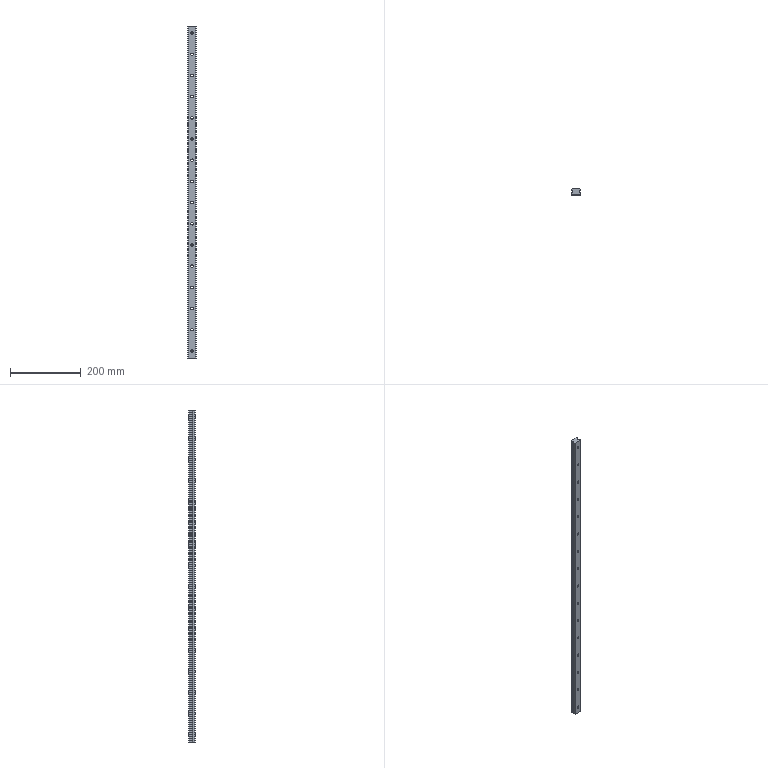Part | STEP file | 0244_Z_004_SX2W33-1240_1 | 1 solid | 97 faces | box 23 x 18 x 940 mm | volume 339429 mm3 | cylinder 69 | plane 28 | commonest cylinder face diameters 7 x32 11 x32 6 x3 3 x2